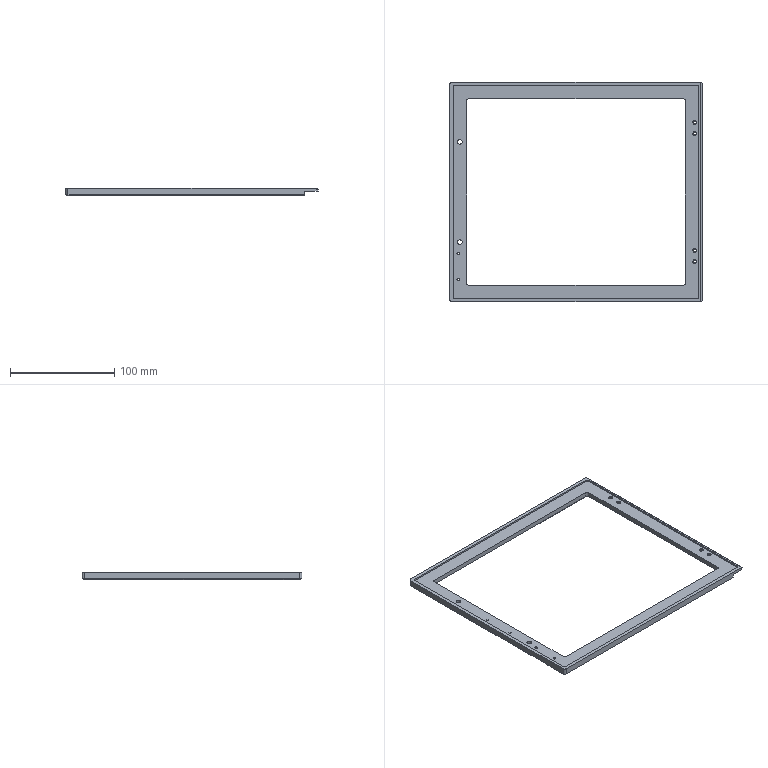NC program | NX | posted with a generic post | part box 241.5 x 210.5 x 7 mm
Lines 3156 to 3179 of 3179:
(PLANAR_MILL_COPY_COPY , TOOL : D6A45)
N6286 T07 M6
N6288 G54
N6290 G17 G0 G90 X123.107 Y105.953 S9500 M3
N6292 G43 Z30. H7
N6294 Z-1.
N6296 G94 G1 Z-2.5 F1250.
N6298 G3 X122.75 Y105.186 R1.
N6300 G1 Y-105.186
N6302 G3 X123.107 Y-105.953 R1.
N6304 G1 Z-1.
N6306 G0 Z30.
N6308 X122.107 Y105.953
N6310 Z-1.
N6312 G1 Z-2.5
N6314 G3 X121.75 Y105.186 R1.
N6316 G1 Y-105.186
N6318 G3 X122.107 Y-105.953 R1.
N6320 G1 Z-1.
N6322 G0 Z30.
N6324 M5
N6326 M2